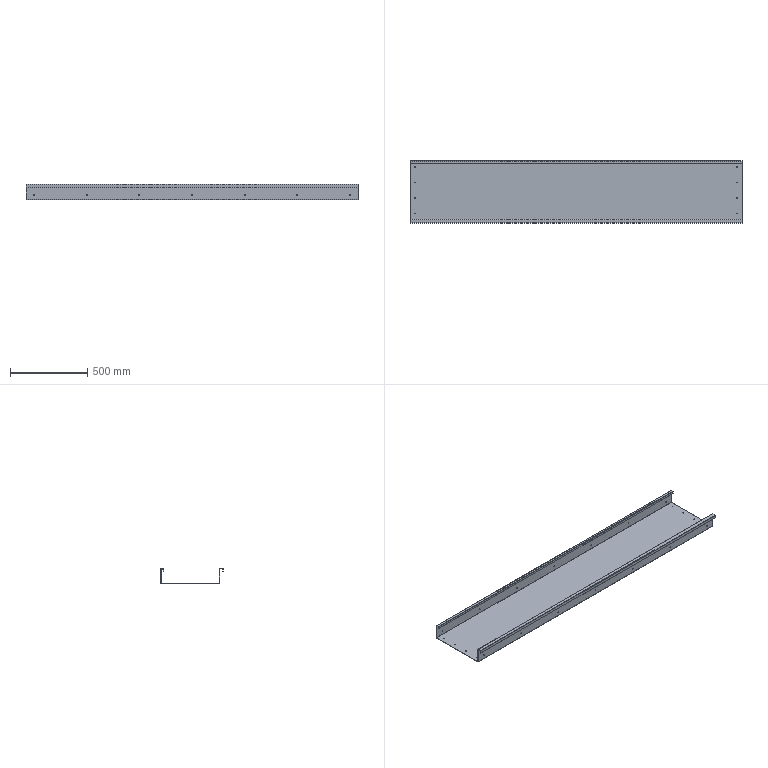Part | STEP file | TS-S14 | 1 solid | 98 faces | box 2145 x 403 x 100 mm | volume 2744257 mm3 | cylinder 56 | plane 42 | commonest cylinder face diameters 5.4 x28 5 x16 0.4 x6 4.4 x6